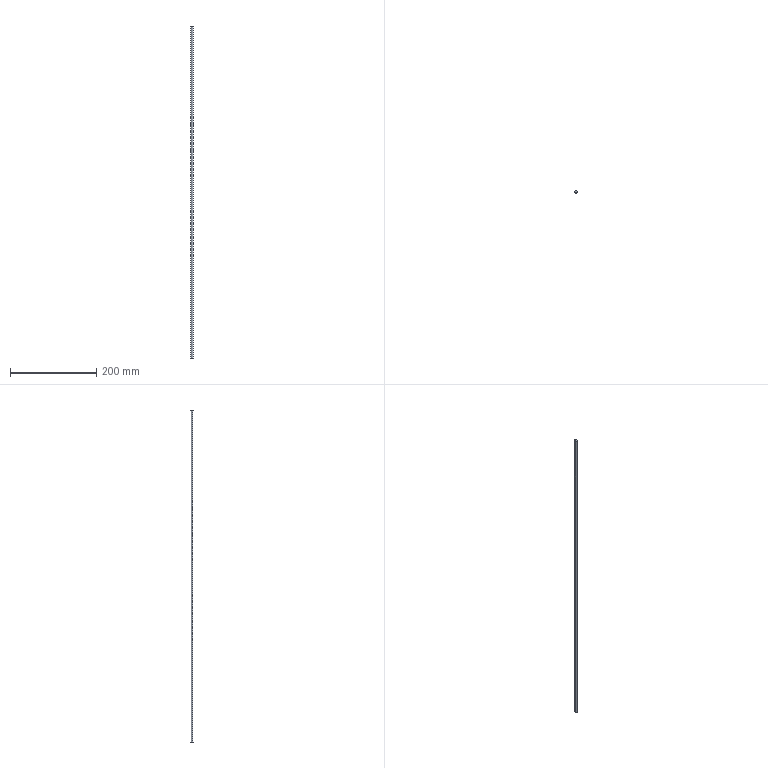Part | SolidWorks | features BaseBody 1 | 1 solid | 4 faces | box 6 x 6 x 768.668 mm | volume 21734 mm3 | cylinder 2 | plane 2 | commonest cylinder face diameters 6 x2
STEP:
#1=CARTESIAN_POINT('',(337.265,269.388,-230.192));
#2=VERTEX_POINT('',#1);
#3=CARTESIAN_POINT('',(343.265,269.388,-230.192));
#4=VERTEX_POINT('',#3);
#5=CARTESIAN_POINT('',(340.265,269.388,-230.192));
#6=DIRECTION('',(0.,0.,-1.));
#7=DIRECTION('',(-1.,0.,0.));
#8=AXIS2_PLACEMENT_3D('',#5,#6,#7);
#9=CIRCLE('',#8,3.);
#10=EDGE_CURVE('',#2,#4,#9,.T.);
#11=ORIENTED_EDGE('',*,*,#10,.F.);
#12=CARTESIAN_POINT('',(337.265,269.388,538.476));
#13=VERTEX_POINT('',#12);
#14=CARTESIAN_POINT('',(337.265,269.388,-230.192));
#15=DIRECTION('',(0.,0.,1.));
#16=VECTOR('',#15,1000.);
#17=LINE('',#14,#16);
#18=EDGE_CURVE('',#2,#13,#17,.T.);
#19=ORIENTED_EDGE('',*,*,#18,.T.);
#20=CARTESIAN_POINT('',(343.265,269.388,538.476));
#21=VERTEX_POINT('',#20);
#22=CARTESIAN_POINT('',(340.265,269.388,538.476));
#23=DIRECTION('',(0.,0.,1.));
#24=DIRECTION('',(-1.,0.,0.));
#25=AXIS2_PLACEMENT_3D('',#22,#23,#24);
#26=CIRCLE('',#25,3.);
#27=EDGE_CURVE('',#21,#13,#26,.T.);
#28=ORIENTED_EDGE('',*,*,#27,.F.);
#29=CARTESIAN_POINT('',(343.265,269.388,-230.192));
#30=DIRECTION('',(0.,0.,1.));
#31=VECTOR('',#30,1000.);
#32=LINE('',#29,#31);
#33=EDGE_CURVE('',#4,#21,#32,.T.);
#34=ORIENTED_EDGE('',*,*,#33,.F.);
#35=EDGE_LOOP('',(#11,#19,#28,#34));
#36=FACE_OUTER_BOUND('',#35,.T.);
#37=CARTESIAN_POINT('',(340.265,269.388,-230.192));
#38=DIRECTION('',(0.,0.,1.));
#39=DIRECTION('',(1.,0.,0.));
#40=AXIS2_PLACEMENT_3D('',#37,#38,#39);
#41=CYLINDRICAL_SURFACE('',#40,3.);
#42=ADVANCED_FACE('',(#36),#41,.T.);
#43=CARTESIAN_POINT('',(340.265,269.388,-230.192));
#44=DIRECTION('',(0.,0.,-1.));
#45=DIRECTION('',(-1.,0.,0.));
#46=AXIS2_PLACEMENT_3D('',#43,#44,#45);
#47=CIRCLE('',#46,3.);
#48=EDGE_CURVE('',#4,#2,#47,.T.);
#49=ORIENTED_EDGE('',*,*,#48,.T.);
#50=ORIENTED_EDGE('',*,*,#10,.T.);
#51=EDGE_LOOP('',(#49,#50));
#52=FACE_OUTER_BOUND('',#51,.T.);
#53=CARTESIAN_POINT('',(340.265,269.388,-230.192));
#54=DIRECTION('',(0.,0.,-1.));
#55=DIRECTION('',(0.,-1.,0.));
#56=AXIS2_PLACEMENT_3D('',#53,#54,#55);
#57=PLANE('',#56);
#58=ADVANCED_FACE('',(#52),#57,.T.);
#59=ORIENTED_EDGE('',*,*,#18,.F.);
#60=ORIENTED_EDGE('',*,*,#48,.F.);
#61=ORIENTED_EDGE('',*,*,#33,.T.);
#62=CARTESIAN_POINT('',(340.265,269.388,538.476));
#63=DIRECTION('',(0.,0.,1.));
#64=DIRECTION('',(-1.,0.,0.));
#65=AXIS2_PLACEMENT_3D('',#62,#63,#64);
#66=CIRCLE('',#65,3.);
#67=EDGE_CURVE('',#13,#21,#66,.T.);
#68=ORIENTED_EDGE('',*,*,#67,.F.);
#69=EDGE_LOOP('',(#59,#60,#61,#68));
#70=FACE_OUTER_BOUND('',#69,.T.);
#71=CARTESIAN_POINT('',(340.265,269.388,-230.192));
#72=DIRECTION('',(0.,0.,1.));
#73=DIRECTION('',(1.,0.,0.));
#74=AXIS2_PLACEMENT_3D('',#71,#72,#73);
#75=CYLINDRICAL_SURFACE('',#74,3.);
#76=ADVANCED_FACE('',(#70),#75,.T.);
#77=ORIENTED_EDGE('',*,*,#27,.T.);
#78=ORIENTED_EDGE('',*,*,#67,.T.);
#79=EDGE_LOOP('',(#77,#78));
#80=FACE_OUTER_BOUND('',#79,.T.);
#81=CARTESIAN_POINT('',(340.265,269.388,538.476));
#82=DIRECTION('',(0.,0.,1.));
#83=DIRECTION('',(1.,0.,0.));
#84=AXIS2_PLACEMENT_3D('',#81,#82,#83);
#85=PLANE('',#84);
#86=ADVANCED_FACE('',(#80),#85,.T.);
#87=CLOSED_SHELL('',(#42,#58,#76,#86));
#88=MANIFOLD_SOLID_BREP('',#87);
#89=CARTESIAN_POINT('',(0.,0.,0.));
#90=DIRECTION('',(0.,0.,1.));
#91=DIRECTION('',(1.,0.,0.));
#92=AXIS2_PLACEMENT_3D('',#89,#90,#91);
#93=(LENGTH_UNIT()NAMED_UNIT(*)SI_UNIT(.MILLI.,.METRE.));
#94=UNCERTAINTY_MEASURE_WITH_UNIT(LENGTH_MEASURE(0.00001),#93,'','');
#95=(NAMED_UNIT(*)PLANE_ANGLE_UNIT()SI_UNIT($,.RADIAN.));
#96=(NAMED_UNIT(*)SI_UNIT($,.STERADIAN.)SOLID_ANGLE_UNIT());
#97=(GEOMETRIC_REPRESENTATION_CONTEXT(3)GLOBAL_UNCERTAINTY_ASSIGNED_CONTEXT((#94))GLOBAL_UNIT_ASSIGNED_CONTEXT((#93,#95,#96))REPRESENTATION_CONTEXT('',''));
#98=ADVANCED_BREP_SHAPE_REPRESENTATION('',(#88,#92),#97);